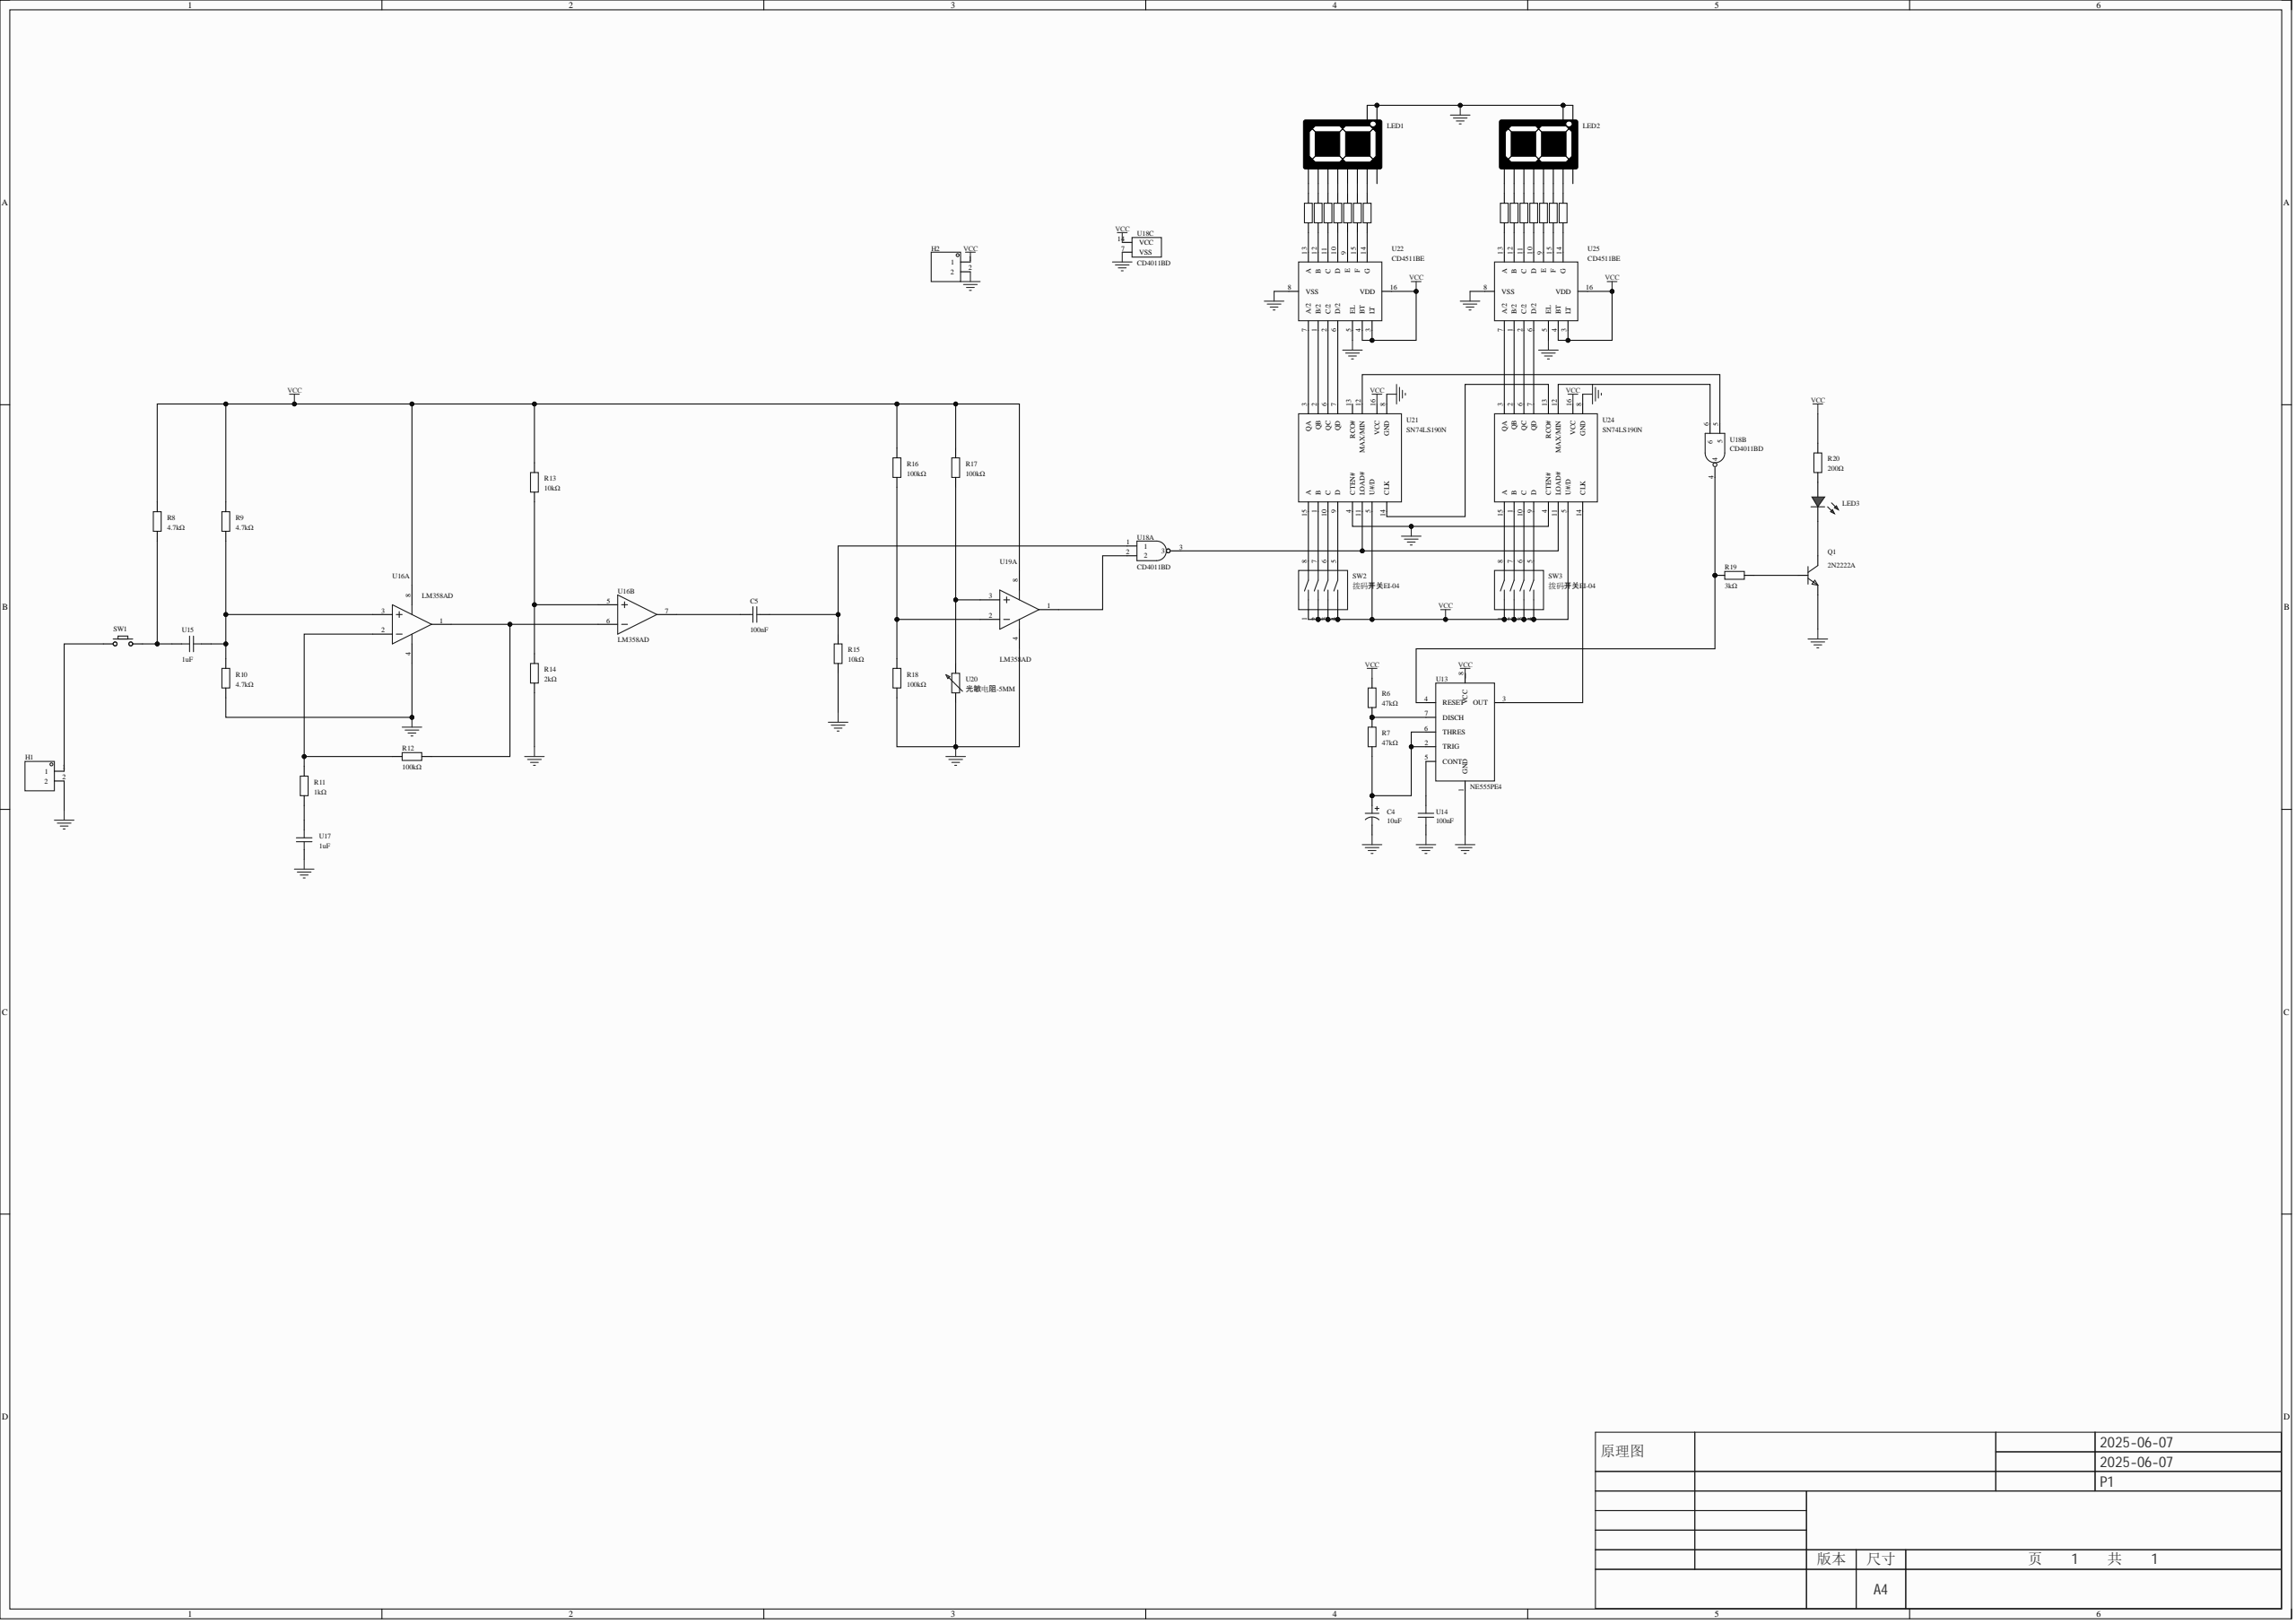Circuit board | Altium Designer | 52 parts | 70 nets
Bill of materials:
Comment,Description,Designator,Footprint,LibRef,Quantity
"10uF","","C4","CAP-TH_BD5.0-P2.00-D0.5-FD","SHG63V10UF03EC0822","1"
"100nF","","C5","CAP-TH_L4.0-W2.5-P2.50-D0.5-A","FA18X7R1H104KNU00","1"
"","","H1, H2","HDR-TH_2P-P2.54-V-M-1","HDR-M_2.54_1x2P","2"
"","","LED1, LED2","LED-SEG-TH_10P-L12.6-W19.0-P2.54-S15.24-BL","LED_SEG_TH_0.56x1","2"
"","","LED3","LED_TH-3mm","LED_TH-R_3mm","1"
"2N2222A","","Q1","TO-92-3_L4.9-W3.7-P1.27-L","2N2222A","1"
"47kΩ","","R6, R7","Res_1/8W","Res_AXIAL-1/8W","2"
"4.7kΩ","","R8, R9, R10","Res_1/8W","Res_AXIAL-1/8W","3"
"1kΩ","","R11","Res_1/8W","Res_AXIAL-1/8W","1"
"100kΩ","","R12, R16, R17, R18","Res_1/8W","Res_AXIAL-1/8W","4"
"10kΩ","","R13, R15, R21, R22, R23, R24, R25, R26, R27, R28, R29, R30, R31, R32, R33, R34","Res_1/8W","Res_AXIAL-1/8W","16"
"2kΩ","","R14","Res_1/8W","Res_AXIAL-1/8W","1"
"3kΩ","","R19","Res_1/8W","Res_AXIAL-1/8W","1"
"200Ω","","R20","Res_1/8W","Res_AXIAL-1/8W","1"
"","","SW1","Key_TH_3.5x6x4.3","Key_TH_3.5x6x4.3","1"
"拨码开关EI-04","","SW2, SW3","SW-TH_DIPSWITCHEI-04","拨码开关EI-04","2"
"NE555PE4","","U13","PDIP-8_L9.6-W6.4-P2.54-LS7.9-BL-1","NE555PE4","1"
"100nF","","U14","CAP-TH_L4.5-W3.0-P2.50-D0.5","FA14X8R1H104KNU00","1"
"1uF","","U15, U17","CAP-TH_L4.0-W2.5-P2.50-D0.5","FA18X7R1E105KRU00","2"
"LM358AD","","U16, U19","SOP-8_L4.9-W3.9-P1.27-LS6.0-BL","LM358AD","2"
"CD4011BD","","U18","PDIP-14_L19.3-W6.4-P2.54-LS7.9-BL-1","CD4011BD","1"
"光敏电阻-5MM","","U20","RES-TH_L4.9-W4.3-P3.4","光敏电阻-5MM","1"
"SN74LS190N","","U21, U24","PDIP-16_L19.2-W6.6-P2.54-LS7.6-BL","SN74LS190N","2"
"CD4511BE","","U22, U25","DIP-16_L19.8-W6.5-P2.54-LS7.6-BL","CD4511BE","2"
Netlist (Protel format):
[
C4
CAP-TH_BD5.0-P2.00-D0.5-FD
10uF



]
[
C5
CAP-TH_L4.0-W2.5-P2.50-D0.5-A
100nF



]
[
H1
HDR-TH_2P-P2.54-V-M-1




]
[
H2
HDR-TH_2P-P2.54-V-M-1




]
[
LED1
LED-SEG-TH_10P-L12.6-W19.0-P2.54-S15.24-BL




]
[
LED2
LED-SEG-TH_10P-L12.6-W19.0-P2.54-S15.24-BL




]
[
LED3
LED_TH-3mm




]
[
Q1
TO-92-3_L4.9-W3.7-P1.27-L
2N2222A



]
[
R6
Res_1/8W
47kΩ



]
[
R7
Res_1/8W
47kΩ



]
[
R8
Res_1/8W
4.7kΩ



]
[
R9
Res_1/8W
4.7kΩ



]
[
R10
Res_1/8W
4.7kΩ



]
[
R11
Res_1/8W
1kΩ



]
[
R12
Res_1/8W
100kΩ



]
[
R13
Res_1/8W
10kΩ



]
[
R14
Res_1/8W
2kΩ



]
[
R15
Res_1/8W
10kΩ



]
[
R16
Res_1/8W
100kΩ



]
[
R17
Res_1/8W
100kΩ



]
[
R18
Res_1/8W
100kΩ



]
[
R19
Res_1/8W
3kΩ



]
[
R20
Res_1/8W
200Ω



]
[
R21
Res_1/8W
10kΩ



]
[
R22
Res_1/8W
10kΩ



]
[
R23
Res_1/8W
10kΩ



]
[
R24
Res_1/8W
10kΩ



]
[
R25
Res_1/8W
10kΩ



]
[
R26
Res_1/8W
10kΩ



]
[
R27
Res_1/8W
10kΩ



]
[
R28
Res_1/8W
10kΩ



]
[
R29
Res_1/8W
10kΩ



]
[
R30
Res_1/8W
10kΩ



]
[
R31
Res_1/8W
10kΩ



]
[
R32
Res_1/8W
10kΩ



]
[
R33
Res_1/8W
10kΩ



]
[
R34
Res_1/8W
10kΩ



]
[
SW1
Key_TH_3.5x6x4.3




]
[
SW2
SW-TH_DIPSWITCHEI-04
拨码开关EI-04



]
[
SW3
SW-TH_DIPSWITCHEI-04
拨码开关EI-04



]
[
U13
PDIP-8_L9.6-W6.4-P2.54-LS7.9-BL-1
NE555PE4



]
[
U14
CAP-TH_L4.5-W3.0-P2.50-D0.5
100nF



]
[
U15
CAP-TH_L4.0-W2.5-P2.50-D0.5
1uF



]
[
U16
SOP-8_L4.9-W3.9-P1.27-LS6.0-BL
LM358AD



]
[
U17
CAP-TH_L4.0-W2.5-P2.50-D0.5
1uF



]
[
U18
PDIP-14_L19.3-W6.4-P2.54-LS7.9-BL-1
CD4011BD



]
[
U19
SOP-8_L4.9-W3.9-P1.27-LS6.0-BL
LM358AD



]
[
U20
RES-TH_L4.9-W4.3-P3.4
光敏电阻-5MM



]
[
U21
PDIP-16_L19.2-W6.6-P2.54-LS7.6-BL
SN74LS190N



]
[
U22
DIP-16_L19.8-W6.5-P2.54-LS7.6-BL
CD4511BE



]
[
U24
PDIP-16_L19.2-W6.6-P2.54-LS7.6-BL
SN74LS190N



]
[
U25
DIP-16_L19.8-W6.5-P2.54-LS7.6-BL
CD4511BE



]
(
VCC
H2-1
R6-2
R8-2
R9-2
R13-2
R16-2
R17-2
R20-2
SW2-1
SW2-2
SW2-3
SW2-4
SW3-1
SW3-2
SW3-3
SW3-4
U13-8
U16-8
U18-14
U19-8
U21-5
U21-16
U22-3
U22-4
U22-16
U24-5
U24-16
U25-3
U25-4
U25-16
)
(
NetU24_7
U24-7
U25-6
)
(
NetU24_6
U24-6
U25-2
)
(
NetU24_3
U24-3
U25-7
)
(
NetU24_2
U24-2
U25-1
)
(
NetU21_14
U21-14
U24-13
)
(
NetU21_7
U21-7
U22-6
)
(
NetU21_6
U21-6
U22-2
)
(
NetU21_3
U21-3
U22-7
)
(
NetU21_2
U21-2
U22-1
)
(
NetU18_6
U18-6
U24-12
)
(
NetU18_5
U18-5
U21-12
)
(
NetU18_3
U18-3
U21-11
U24-11
)
(
NetU18_2
U18-2
U19-1
)
(
NetU13_5
U13-5
U14-2
)
(
NetU13_3
U13-3
U24-14
)
(
NetSW3_8
SW3-8
U24-15
)
(
NetSW3_7
SW3-7
U24-1
)
(
NetSW3_6
SW3-6
U24-10
)
(
NetSW3_5
SW3-5
U24-9
)
(
NetSW2_8
SW2-8
U21-15
)
(
NetSW2_7
SW2-7
U21-1
)
(
NetSW2_6
SW2-6
U21-10
)
(
NetSW2_5
SW2-5
U21-9
)
(
NetR34_1
R34-1
U25-14
)
(
NetR33_1
R33-1
U25-15
)
(
NetR32_1
R32-1
U25-9
)
(
NetR31_1
R31-1
U25-10
)
(
NetR30_1
R30-1
U25-11
)
(
NetR29_1
R29-1
U25-12
)
(
NetR28_1
R28-1
U25-13
)
(
NetR27_1
R27-1
U22-14
)
(
NetR26_1
R26-1
U22-15
)
(
NetR25_1
R25-1
U22-9
)
(
NetR24_1
R24-1
U22-10
)
(
NetR23_1
R23-1
U22-11
)
(
NetR22_1
R22-1
U22-12
)
(
NetR21_1
R21-1
U22-13
)
(
NetR19_2
R19-2
U13-4
U18-4
)
(
NetR17_1
R17-1
U19-3
U20-2
)
(
NetR16_1
R16-1
R18-2
U19-2
)
(
NetR13_1
R13-1
R14-2
U16-5
)
(
NetR12_2
R12-2
U16-1
U16-6
)
(
NetR11_2
R11-2
R12-1
U16-2
)
(
NetR11_1
R11-1
U17-2
)
(
NetR9_1
R9-1
R10-2
U15-2
U16-3
)
(
NetR8_1
R8-1
SW1-B
U15-1
)
(
NetR6_1
R6-1
R7-2
U13-7
)
(
NetQ1_2
Q1-2
R19-1
)
(
NetLED3_2
LED3-2
Q1-3
)
(
NetLED3_1
LED3-1
R20-1
)
(
NetLED2_10
LED2-10
R34-2
)
(
NetLED2_9
LED2-9
R33-2
)
(
NetLED2_7
LED2-7
R28-2
)
(
NetLED2_6
LED2-6
R29-2
)
(
NetLED2_4
LED2-4
R30-2
)
(
NetLED2_2
LED2-2
R31-2
)
(
NetLED2_1
LED2-1
R32-2
)
(
NetLED1_10
LED1-10
R27-2
)
(
NetLED1_9
LED1-9
R26-2
)
(
NetLED1_7
LED1-7
R21-2
)
(
NetLED1_6
LED1-6
R22-2
)
(
NetLED1_4
LED1-4
R23-2
)
(
NetLED1_2
LED1-2
R24-2
)
(
NetLED1_1
LED1-1
R25-2
)
(
NetH1_1
H1-1
SW1-A
)
(
NetC5_2
C5-2
R15-2
U18-1
)
(
NetC5_1
C5-1
U16-7
)
(
NetC4_1
C4-1
R7-1
U13-2
U13-6
)
(
GND
C4-2
H1-2
H2-2
LED1-3
LED1-8
LED2-3
LED2-8
Q1-1
R10-1
R14-1
R15-1
R18-1
U13-1
U14-1
U16-4
U17-1
U18-7
U19-4
U20-1
U21-4
U21-8
U22-5
U22-8
U24-4
U24-8
U25-5
U25-8
)